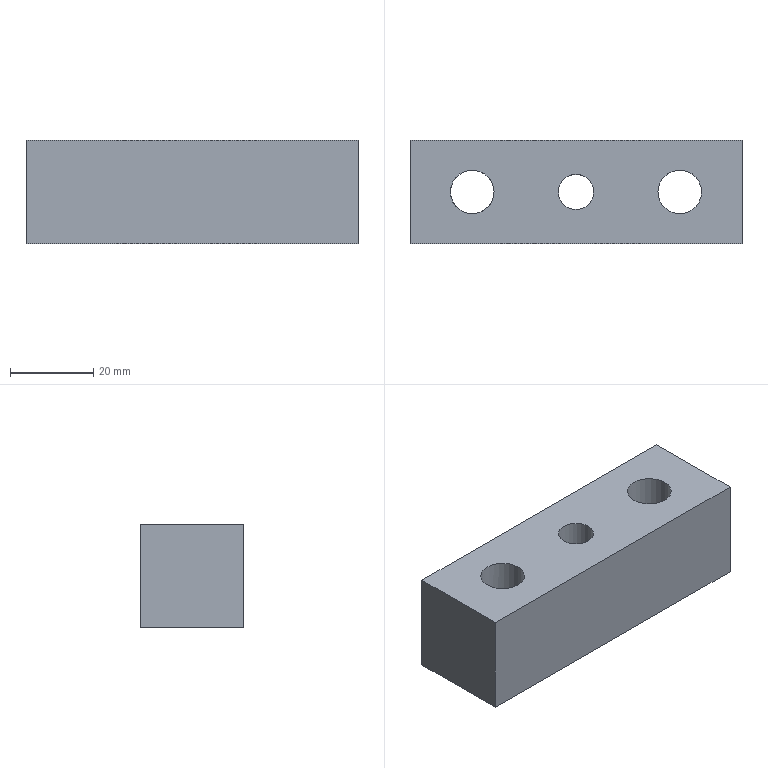Part | STEP file | 1_id1362_x_t | 1 solid | 15 faces | box 80 x 25 x 25 mm | volume 39657 mm3 | plane 9 | cylinder 6 | commonest cylinder face diameters 10.5 x2 17 x2 8.5 x1 11 x1
STEP:
#1=CARTESIAN_POINT('',(0.,0.,0.));
#2=DIRECTION('',(0.,0.,1.));
#3=DIRECTION('',(1.,0.,0.));
#4=AXIS2_PLACEMENT_3D('',#1,#2,#3);
#5=CARTESIAN_POINT('',(752.176,377.474,113.61));
#6=VERTEX_POINT('',#5);
#7=CARTESIAN_POINT('',(747.926,377.474,113.61));
#8=DIRECTION('',(0.,0.,-1.));
#9=DIRECTION('',(1.,0.,0.));
#10=AXIS2_PLACEMENT_3D('',#7,#8,#9);
#11=CIRCLE('',#10,4.25);
#12=CARTESIAN_POINT('',(747.926,377.474,117.86));
#13=DIRECTION('',(0.,0.,1.));
#14=DIRECTION('',(1.,0.,0.));
#15=AXIS2_PLACEMENT_3D('',#12,#13,#14);
#16=CYLINDRICAL_SURFACE('',#15,4.25);
#17=CARTESIAN_POINT('',(6.283,-4.25));
#18=DIRECTION('',(-1.,0.));
#19=VECTOR('',#18,1.);
#20=LINE('',#17,#19);
#21=(GEOMETRIC_REPRESENTATION_CONTEXT(2)PARAMETRIC_REPRESENTATION_CONTEXT()REPRESENTATION_CONTEXT('',''));
#22=DEFINITIONAL_REPRESENTATION('',(#20),#21);
#23=PCURVE('',#16,#22);
#24=CARTESIAN_POINT('',(707.926,389.974,113.61));
#25=DIRECTION('',(0.,0.,-1.));
#26=DIRECTION('',(-1.,0.,0.));
#27=AXIS2_PLACEMENT_3D('',#24,#25,#26);
#28=PLANE('',#27);
#29=CARTESIAN_POINT('',(-40.,-12.5));
#30=DIRECTION('',(-1.,0.));
#31=AXIS2_PLACEMENT_2D('',#29,#30);
#32=CIRCLE('',#31,4.25);
#33=(GEOMETRIC_REPRESENTATION_CONTEXT(2)PARAMETRIC_REPRESENTATION_CONTEXT()REPRESENTATION_CONTEXT('',''));
#34=DEFINITIONAL_REPRESENTATION('',(#32),#33);
#35=PCURVE('',#28,#34);
#36=SURFACE_CURVE('',#11,(#23,#35),.PCURVE_S1.);
#37=EDGE_CURVE('',#6,#6,#36,.T.);
#38=ORIENTED_EDGE('',*,*,#37,.T.);
#39=CARTESIAN_POINT('',(752.176,377.474,98.61));
#40=VERTEX_POINT('',#39);
#41=CARTESIAN_POINT('',(752.176,377.474,98.61));
#42=CARTESIAN_POINT('',(752.176,377.474,113.61));
#43=B_SPLINE_CURVE_WITH_KNOTS('',1,(#41,#42),.UNSPECIFIED.,.F.,.F.,(2,2),(-19.25,-4.25),.PIECEWISE_BEZIER_KNOTS.);
#44=CARTESIAN_POINT('',(0.,0.));
#45=DIRECTION('',(0.,1.));
#46=VECTOR('',#45,1.);
#47=LINE('',#44,#46);
#48=(GEOMETRIC_REPRESENTATION_CONTEXT(2)PARAMETRIC_REPRESENTATION_CONTEXT()REPRESENTATION_CONTEXT('',''));
#49=DEFINITIONAL_REPRESENTATION('',(#47),#48);
#50=PCURVE('',#16,#49);
#51=CARTESIAN_POINT('',(6.283,0.));
#52=DIRECTION('',(0.,1.));
#53=VECTOR('',#52,1.);
#54=LINE('',#51,#53);
#55=(GEOMETRIC_REPRESENTATION_CONTEXT(2)PARAMETRIC_REPRESENTATION_CONTEXT()REPRESENTATION_CONTEXT('',''));
#56=DEFINITIONAL_REPRESENTATION('',(#54),#55);
#57=PCURVE('',#16,#56);
#58=SEAM_CURVE('',#43,(#50,#57),.PCURVE_S1.);
#59=EDGE_CURVE('',#40,#6,#58,.T.);
#60=ORIENTED_EDGE('',*,*,#59,.F.);
#61=CARTESIAN_POINT('',(743.676,377.474,98.61));
#62=VERTEX_POINT('',#61);
#63=CARTESIAN_POINT('',(747.926,377.474,98.61));
#64=DIRECTION('',(0.,0.,1.));
#65=DIRECTION('',(-1.,0.,0.));
#66=AXIS2_PLACEMENT_3D('',#63,#64,#65);
#67=CIRCLE('',#66,4.25);
#68=CARTESIAN_POINT('',(-3.142,-19.25));
#69=DIRECTION('',(1.,0.));
#70=VECTOR('',#69,1.);
#71=LINE('',#68,#70);
#72=(GEOMETRIC_REPRESENTATION_CONTEXT(2)PARAMETRIC_REPRESENTATION_CONTEXT()REPRESENTATION_CONTEXT('',''));
#73=DEFINITIONAL_REPRESENTATION('',(#71),#72);
#74=PCURVE('',#16,#73);
#75=CARTESIAN_POINT('',(747.926,377.474,98.61));
#76=DIRECTION('',(0.,0.,-1.));
#77=DIRECTION('',(-1.,0.,0.));
#78=AXIS2_PLACEMENT_3D('',#75,#76,#77);
#79=PLANE('',#78);
#80=CARTESIAN_POINT('',(4.25,0.));
#81=CARTESIAN_POINT('',(4.25,-7.361));
#82=CARTESIAN_POINT('',(-2.125,-3.681));
#83=CARTESIAN_POINT('',(-8.5,0.));
#84=CARTESIAN_POINT('',(-2.125,3.681));
#85=CARTESIAN_POINT('',(4.25,7.361));
#86=CARTESIAN_POINT('',(4.25,0.));
#87=(BOUNDED_CURVE()B_SPLINE_CURVE(2,(#80,#81,#82,#83,#84,#85,#86),.UNSPECIFIED.,.T.,.F.)B_SPLINE_CURVE_WITH_KNOTS((1,2,2,2,2,1),(-2.094,0.,2.094,4.189,6.283,8.378),.UNSPECIFIED.)CURVE()GEOMETRIC_REPRESENTATION_ITEM()RATIONAL_B_SPLINE_CURVE((1.,0.5,1.,0.5,1.,0.5,1.))REPRESENTATION_ITEM(''));
#88=(GEOMETRIC_REPRESENTATION_CONTEXT(2)PARAMETRIC_REPRESENTATION_CONTEXT()REPRESENTATION_CONTEXT('',''));
#89=DEFINITIONAL_REPRESENTATION('',(#87),#88);
#90=PCURVE('',#79,#89);
#91=SURFACE_CURVE('',#67,(#74,#90),.PCURVE_S1.);
#92=EDGE_CURVE('',#40,#62,#91,.T.);
#93=ORIENTED_EDGE('',*,*,#92,.T.);
#94=CARTESIAN_POINT('',(747.926,377.474,98.61));
#95=DIRECTION('',(0.,0.,1.));
#96=DIRECTION('',(-1.,0.,0.));
#97=AXIS2_PLACEMENT_3D('',#94,#95,#96);
#98=CIRCLE('',#97,4.25);
#99=CARTESIAN_POINT('',(3.142,-19.25));
#100=DIRECTION('',(1.,0.));
#101=VECTOR('',#100,1.);
#102=LINE('',#99,#101);
#103=(GEOMETRIC_REPRESENTATION_CONTEXT(2)PARAMETRIC_REPRESENTATION_CONTEXT()REPRESENTATION_CONTEXT('',''));
#104=DEFINITIONAL_REPRESENTATION('',(#102),#103);
#105=PCURVE('',#16,#104);
#106=CARTESIAN_POINT('',(4.25,0.));
#107=CARTESIAN_POINT('',(4.25,-7.361));
#108=CARTESIAN_POINT('',(-2.125,-3.681));
#109=CARTESIAN_POINT('',(-8.5,0.));
#110=CARTESIAN_POINT('',(-2.125,3.681));
#111=CARTESIAN_POINT('',(4.25,7.361));
#112=CARTESIAN_POINT('',(4.25,0.));
#113=(BOUNDED_CURVE()B_SPLINE_CURVE(2,(#106,#107,#108,#109,#110,#111,#112),.UNSPECIFIED.,.T.,.F.)B_SPLINE_CURVE_WITH_KNOTS((1,2,2,2,2,1),(-2.094,0.,2.094,4.189,6.283,8.378),.UNSPECIFIED.)CURVE()GEOMETRIC_REPRESENTATION_ITEM()RATIONAL_B_SPLINE_CURVE((1.,0.5,1.,0.5,1.,0.5,1.))REPRESENTATION_ITEM(''));
#114=(GEOMETRIC_REPRESENTATION_CONTEXT(2)PARAMETRIC_REPRESENTATION_CONTEXT()REPRESENTATION_CONTEXT('',''));
#115=DEFINITIONAL_REPRESENTATION('',(#113),#114);
#116=PCURVE('',#79,#115);
#117=SURFACE_CURVE('',#98,(#105,#116),.PCURVE_S1.);
#118=EDGE_CURVE('',#62,#40,#117,.T.);
#119=ORIENTED_EDGE('',*,*,#118,.T.);
#120=ORIENTED_EDGE('',*,*,#59,.T.);
#121=EDGE_LOOP('',(#38,#60,#93,#119,#120));
#122=FACE_BOUND('',#121,.F.);
#123=ADVANCED_FACE('',(#122),#16,.F.);
#124=CARTESIAN_POINT('',(707.926,364.974,113.61));
#125=VERTEX_POINT('',#124);
#126=CARTESIAN_POINT('',(787.926,364.974,113.61));
#127=VERTEX_POINT('',#126);
#128=CARTESIAN_POINT('',(707.926,364.974,113.61));
#129=DIRECTION('',(1.,0.,0.));
#130=VECTOR('',#129,1.);
#131=LINE('',#128,#130);
#132=CARTESIAN_POINT('',(0.,-25.));
#133=DIRECTION('',(-1.,0.));
#134=VECTOR('',#133,1.);
#135=LINE('',#132,#134);
#136=(GEOMETRIC_REPRESENTATION_CONTEXT(2)PARAMETRIC_REPRESENTATION_CONTEXT()REPRESENTATION_CONTEXT('',''));
#137=DEFINITIONAL_REPRESENTATION('',(#135),#136);
#138=PCURVE('',#28,#137);
#139=CARTESIAN_POINT('',(787.926,364.974,113.61));
#140=DIRECTION('',(0.,-1.,0.));
#141=DIRECTION('',(-1.,0.,0.));
#142=AXIS2_PLACEMENT_3D('',#139,#140,#141);
#143=PLANE('',#142);
#144=CARTESIAN_POINT('',(80.,0.));
#145=DIRECTION('',(-1.,0.));
#146=VECTOR('',#145,1.);
#147=LINE('',#144,#146);
#148=(GEOMETRIC_REPRESENTATION_CONTEXT(2)PARAMETRIC_REPRESENTATION_CONTEXT()REPRESENTATION_CONTEXT('',''));
#149=DEFINITIONAL_REPRESENTATION('',(#147),#148);
#150=PCURVE('',#143,#149);
#151=SURFACE_CURVE('',#131,(#138,#150),.PCURVE_S1.);
#152=EDGE_CURVE('',#125,#127,#151,.T.);
#153=ORIENTED_EDGE('',*,*,#152,.T.);
#154=CARTESIAN_POINT('',(787.926,389.974,113.61));
#155=VERTEX_POINT('',#154);
#156=CARTESIAN_POINT('',(787.926,364.974,113.61));
#157=DIRECTION('',(0.,1.,0.));
#158=VECTOR('',#157,1.);
#159=LINE('',#156,#158);
#160=CARTESIAN_POINT('',(-80.,-25.));
#161=DIRECTION('',(0.,1.));
#162=VECTOR('',#161,1.);
#163=LINE('',#160,#162);
#164=(GEOMETRIC_REPRESENTATION_CONTEXT(2)PARAMETRIC_REPRESENTATION_CONTEXT()REPRESENTATION_CONTEXT('',''));
#165=DEFINITIONAL_REPRESENTATION('',(#163),#164);
#166=PCURVE('',#28,#165);
#167=CARTESIAN_POINT('',(787.926,389.974,113.61));
#168=DIRECTION('',(1.,0.,0.));
#169=DIRECTION('',(0.,1.,0.));
#170=AXIS2_PLACEMENT_3D('',#167,#168,#169);
#171=PLANE('',#170);
#172=CARTESIAN_POINT('',(-25.,0.));
#173=DIRECTION('',(1.,0.));
#174=VECTOR('',#173,1.);
#175=LINE('',#172,#174);
#176=(GEOMETRIC_REPRESENTATION_CONTEXT(2)PARAMETRIC_REPRESENTATION_CONTEXT()REPRESENTATION_CONTEXT('',''));
#177=DEFINITIONAL_REPRESENTATION('',(#175),#176);
#178=PCURVE('',#171,#177);
#179=SURFACE_CURVE('',#159,(#166,#178),.PCURVE_S1.);
#180=EDGE_CURVE('',#127,#155,#179,.T.);
#181=ORIENTED_EDGE('',*,*,#180,.T.);
#182=CARTESIAN_POINT('',(707.926,389.974,113.61));
#183=VERTEX_POINT('',#182);
#184=CARTESIAN_POINT('',(787.926,389.974,113.61));
#185=DIRECTION('',(-1.,0.,0.));
#186=VECTOR('',#185,1.);
#187=LINE('',#184,#186);
#188=CARTESIAN_POINT('',(-80.,0.));
#189=DIRECTION('',(1.,0.));
#190=VECTOR('',#189,1.);
#191=LINE('',#188,#190);
#192=(GEOMETRIC_REPRESENTATION_CONTEXT(2)PARAMETRIC_REPRESENTATION_CONTEXT()REPRESENTATION_CONTEXT('',''));
#193=DEFINITIONAL_REPRESENTATION('',(#191),#192);
#194=PCURVE('',#28,#193);
#195=CARTESIAN_POINT('',(707.926,389.974,113.61));
#196=DIRECTION('',(0.,1.,0.));
#197=DIRECTION('',(0.,0.,-1.));
#198=AXIS2_PLACEMENT_3D('',#195,#196,#197);
#199=PLANE('',#198);
#200=CARTESIAN_POINT('',(0.,-80.));
#201=DIRECTION('',(0.,1.));
#202=VECTOR('',#201,1.);
#203=LINE('',#200,#202);
#204=(GEOMETRIC_REPRESENTATION_CONTEXT(2)PARAMETRIC_REPRESENTATION_CONTEXT()REPRESENTATION_CONTEXT('',''));
#205=DEFINITIONAL_REPRESENTATION('',(#203),#204);
#206=PCURVE('',#199,#205);
#207=SURFACE_CURVE('',#187,(#194,#206),.PCURVE_S1.);
#208=EDGE_CURVE('',#155,#183,#207,.T.);
#209=ORIENTED_EDGE('',*,*,#208,.T.);
#210=CARTESIAN_POINT('',(707.926,389.974,113.61));
#211=DIRECTION('',(0.,-1.,0.));
#212=VECTOR('',#211,1.);
#213=LINE('',#210,#212);
#214=CARTESIAN_POINT('',(0.,0.));
#215=DIRECTION('',(0.,-1.));
#216=VECTOR('',#215,1.);
#217=LINE('',#214,#216);
#218=(GEOMETRIC_REPRESENTATION_CONTEXT(2)PARAMETRIC_REPRESENTATION_CONTEXT()REPRESENTATION_CONTEXT('',''));
#219=DEFINITIONAL_REPRESENTATION('',(#217),#218);
#220=PCURVE('',#28,#219);
#221=CARTESIAN_POINT('',(707.926,364.974,113.61));
#222=DIRECTION('',(-1.,0.,0.));
#223=DIRECTION('',(0.,0.,1.));
#224=AXIS2_PLACEMENT_3D('',#221,#222,#223);
#225=PLANE('',#224);
#226=CARTESIAN_POINT('',(0.,25.));
#227=DIRECTION('',(0.,-1.));
#228=VECTOR('',#227,1.);
#229=LINE('',#226,#228);
#230=(GEOMETRIC_REPRESENTATION_CONTEXT(2)PARAMETRIC_REPRESENTATION_CONTEXT()REPRESENTATION_CONTEXT('',''));
#231=DEFINITIONAL_REPRESENTATION('',(#229),#230);
#232=PCURVE('',#225,#231);
#233=SURFACE_CURVE('',#213,(#220,#232),.PCURVE_S1.);
#234=EDGE_CURVE('',#183,#125,#233,.T.);
#235=ORIENTED_EDGE('',*,*,#234,.T.);
#236=EDGE_LOOP('',(#153,#181,#209,#235));
#237=FACE_BOUND('',#236,.T.);
#238=CARTESIAN_POINT('',(728.176,377.474,113.61));
#239=VERTEX_POINT('',#238);
#240=CARTESIAN_POINT('',(722.926,377.474,113.61));
#241=DIRECTION('',(0.,0.,-1.));
#242=DIRECTION('',(1.,0.,0.));
#243=AXIS2_PLACEMENT_3D('',#240,#241,#242);
#244=CIRCLE('',#243,5.25);
#245=CARTESIAN_POINT('',(-15.,-12.5));
#246=DIRECTION('',(-1.,0.));
#247=AXIS2_PLACEMENT_2D('',#245,#246);
#248=CIRCLE('',#247,5.25);
#249=(GEOMETRIC_REPRESENTATION_CONTEXT(2)PARAMETRIC_REPRESENTATION_CONTEXT()REPRESENTATION_CONTEXT('',''));
#250=DEFINITIONAL_REPRESENTATION('',(#248),#249);
#251=PCURVE('',#28,#250);
#252=CARTESIAN_POINT('',(722.926,377.474,113.86));
#253=DIRECTION('',(0.,0.,1.));
#254=DIRECTION('',(0.,1.,0.));
#255=AXIS2_PLACEMENT_3D('',#252,#253,#254);
#256=CYLINDRICAL_SURFACE('',#255,5.25);
#257=CARTESIAN_POINT('',(10.996,-0.25));
#258=DIRECTION('',(-1.,0.));
#259=VECTOR('',#258,1.);
#260=LINE('',#257,#259);
#261=(GEOMETRIC_REPRESENTATION_CONTEXT(2)PARAMETRIC_REPRESENTATION_CONTEXT()REPRESENTATION_CONTEXT('',''));
#262=DEFINITIONAL_REPRESENTATION('',(#260),#261);
#263=PCURVE('',#256,#262);
#264=SURFACE_CURVE('',#244,(#251,#263),.PCURVE_S1.);
#265=EDGE_CURVE('',#239,#239,#264,.T.);
#266=ORIENTED_EDGE('',*,*,#265,.T.);
#267=EDGE_LOOP('',(#266));
#268=FACE_BOUND('',#267,.T.);
#269=ORIENTED_EDGE('',*,*,#37,.T.);
#270=EDGE_LOOP('',(#269));
#271=FACE_BOUND('',#270,.T.);
#272=CARTESIAN_POINT('',(778.176,377.474,113.61));
#273=VERTEX_POINT('',#272);
#274=CARTESIAN_POINT('',(772.926,377.474,113.61));
#275=DIRECTION('',(0.,0.,-1.));
#276=DIRECTION('',(1.,0.,0.));
#277=AXIS2_PLACEMENT_3D('',#274,#275,#276);
#278=CIRCLE('',#277,5.25);
#279=CARTESIAN_POINT('',(-65.,-12.5));
#280=DIRECTION('',(-1.,0.));
#281=AXIS2_PLACEMENT_2D('',#279,#280);
#282=CIRCLE('',#281,5.25);
#283=(GEOMETRIC_REPRESENTATION_CONTEXT(2)PARAMETRIC_REPRESENTATION_CONTEXT()REPRESENTATION_CONTEXT('',''));
#284=DEFINITIONAL_REPRESENTATION('',(#282),#283);
#285=PCURVE('',#28,#284);
#286=CARTESIAN_POINT('',(772.926,377.474,113.86));
#287=DIRECTION('',(0.,0.,1.));
#288=DIRECTION('',(0.,1.,0.));
#289=AXIS2_PLACEMENT_3D('',#286,#287,#288);
#290=CYLINDRICAL_SURFACE('',#289,5.25);
#291=CARTESIAN_POINT('',(10.996,-0.25));
#292=DIRECTION('',(-1.,0.));
#293=VECTOR('',#292,1.);
#294=LINE('',#291,#293);
#295=(GEOMETRIC_REPRESENTATION_CONTEXT(2)PARAMETRIC_REPRESENTATION_CONTEXT()REPRESENTATION_CONTEXT('',''));
#296=DEFINITIONAL_REPRESENTATION('',(#294),#295);
#297=PCURVE('',#290,#296);
#298=SURFACE_CURVE('',#278,(#285,#297),.PCURVE_S1.);
#299=EDGE_CURVE('',#273,#273,#298,.T.);
#300=ORIENTED_EDGE('',*,*,#299,.T.);
#301=EDGE_LOOP('',(#300));
#302=FACE_BOUND('',#301,.T.);
#303=ADVANCED_FACE('',(#237,#268,#271,#302),#28,.F.);
#304=ORIENTED_EDGE('',*,*,#265,.T.);
#305=CARTESIAN_POINT('',(728.176,377.474,103.61));
#306=VERTEX_POINT('',#305);
#307=CARTESIAN_POINT('',(728.176,377.474,103.61));
#308=CARTESIAN_POINT('',(728.176,377.474,113.61));
#309=B_SPLINE_CURVE_WITH_KNOTS('',1,(#307,#308),.UNSPECIFIED.,.F.,.F.,(2,2),(-10.25,-0.25),.PIECEWISE_BEZIER_KNOTS.);
#310=CARTESIAN_POINT('',(4.712,0.));
#311=DIRECTION('',(0.,1.));
#312=VECTOR('',#311,1.);
#313=LINE('',#310,#312);
#314=(GEOMETRIC_REPRESENTATION_CONTEXT(2)PARAMETRIC_REPRESENTATION_CONTEXT()REPRESENTATION_CONTEXT('',''));
#315=DEFINITIONAL_REPRESENTATION('',(#313),#314);
#316=PCURVE('',#256,#315);
#317=CARTESIAN_POINT('',(10.996,0.));
#318=DIRECTION('',(0.,1.));
#319=VECTOR('',#318,1.);
#320=LINE('',#317,#319);
#321=(GEOMETRIC_REPRESENTATION_CONTEXT(2)PARAMETRIC_REPRESENTATION_CONTEXT()REPRESENTATION_CONTEXT('',''));
#322=DEFINITIONAL_REPRESENTATION('',(#320),#321);
#323=PCURVE('',#256,#322);
#324=SEAM_CURVE('',#309,(#316,#323),.PCURVE_S1.);
#325=EDGE_CURVE('',#306,#239,#324,.T.);
#326=ORIENTED_EDGE('',*,*,#325,.F.);
#327=CARTESIAN_POINT('',(722.926,372.224,103.61));
#328=VERTEX_POINT('',#327);
#329=CARTESIAN_POINT('',(722.926,377.474,103.61));
#330=DIRECTION('',(0.,0.,1.));
#331=DIRECTION('',(0.,-1.,0.));
#332=AXIS2_PLACEMENT_3D('',#329,#330,#331);
#333=CIRCLE('',#332,5.25);
#334=CARTESIAN_POINT('',(3.142,-10.25));
#335=DIRECTION('',(1.,0.));
#336=VECTOR('',#335,1.);
#337=LINE('',#334,#336);
#338=(GEOMETRIC_REPRESENTATION_CONTEXT(2)PARAMETRIC_REPRESENTATION_CONTEXT()REPRESENTATION_CONTEXT('',''));
#339=DEFINITIONAL_REPRESENTATION('',(#337),#338);
#340=PCURVE('',#256,#339);
#341=CARTESIAN_POINT('',(722.926,377.474,103.61));
#342=DIRECTION('',(0.,0.,1.));
#343=DIRECTION('',(0.,-1.,0.));
#344=AXIS2_PLACEMENT_3D('',#341,#342,#343);
#345=PLANE('',#344);
#346=CARTESIAN_POINT('',(0.,0.));
#347=DIRECTION('',(1.,0.));
#348=AXIS2_PLACEMENT_2D('',#346,#347);
#349=CIRCLE('',#348,5.25);
#350=(GEOMETRIC_REPRESENTATION_CONTEXT(2)PARAMETRIC_REPRESENTATION_CONTEXT()REPRESENTATION_CONTEXT('',''));
#351=DEFINITIONAL_REPRESENTATION('',(#349),#350);
#352=PCURVE('',#345,#351);
#353=SURFACE_CURVE('',#333,(#340,#352),.PCURVE_S1.);
#354=EDGE_CURVE('',#306,#328,#353,.T.);
#355=ORIENTED_EDGE('',*,*,#354,.T.);
#356=CARTESIAN_POINT('',(722.926,377.474,103.61));
#357=DIRECTION('',(0.,0.,1.));
#358=DIRECTION('',(0.,-1.,0.));
#359=AXIS2_PLACEMENT_3D('',#356,#357,#358);
#360=CIRCLE('',#359,5.25);
#361=CARTESIAN_POINT('',(9.425,-10.25));
#362=DIRECTION('',(1.,0.));
#363=VECTOR('',#362,1.);
#364=LINE('',#361,#363);
#365=(GEOMETRIC_REPRESENTATION_CONTEXT(2)PARAMETRIC_REPRESENTATION_CONTEXT()REPRESENTATION_CONTEXT('',''));
#366=DEFINITIONAL_REPRESENTATION('',(#364),#365);
#367=PCURVE('',#256,#366);
#368=CARTESIAN_POINT('',(0.,0.));
#369=DIRECTION('',(1.,0.));
#370=AXIS2_PLACEMENT_2D('',#368,#369);
#371=CIRCLE('',#370,5.25);
#372=(GEOMETRIC_REPRESENTATION_CONTEXT(2)PARAMETRIC_REPRESENTATION_CONTEXT()REPRESENTATION_CONTEXT('',''));
#373=DEFINITIONAL_REPRESENTATION('',(#371),#372);
#374=PCURVE('',#345,#373);
#375=SURFACE_CURVE('',#360,(#367,#374),.PCURVE_S1.);
#376=EDGE_CURVE('',#328,#306,#375,.T.);
#377=ORIENTED_EDGE('',*,*,#376,.T.);
#378=ORIENTED_EDGE('',*,*,#325,.T.);
#379=EDGE_LOOP('',(#304,#326,#355,#377,#378));
#380=FACE_BOUND('',#379,.F.);
#381=ADVANCED_FACE('',(#380),#256,.F.);
#382=CARTESIAN_POINT('',(722.926,368.974,103.61));
#383=VERTEX_POINT('',#382);
#384=CARTESIAN_POINT('',(722.926,385.974,103.61));
#385=VERTEX_POINT('',#384);
#386=CARTESIAN_POINT('',(722.926,377.474,103.61));
#387=DIRECTION('',(0.,0.,-1.));
#388=DIRECTION('',(0.,-1.,0.));
#389=AXIS2_PLACEMENT_3D('',#386,#387,#388);
#390=CIRCLE('',#389,8.5);
#391=CARTESIAN_POINT('',(8.5,0.));
#392=CARTESIAN_POINT('',(8.5,-14.722));
#393=CARTESIAN_POINT('',(-4.25,-7.361));
#394=CARTESIAN_POINT('',(-17.,0.));
#395=CARTESIAN_POINT('',(-4.25,7.361));
#396=CARTESIAN_POINT('',(8.5,14.722));
#397=CARTESIAN_POINT('',(8.5,0.));
#398=(BOUNDED_CURVE()B_SPLINE_CURVE(2,(#391,#392,#393,#394,#395,#396,#397),.UNSPECIFIED.,.T.,.F.)B_SPLINE_CURVE_WITH_KNOTS((1,2,2,2,2,1),(-2.094,0.,2.094,4.189,6.283,8.378),.UNSPECIFIED.)CURVE()GEOMETRIC_REPRESENTATION_ITEM()RATIONAL_B_SPLINE_CURVE((1.,0.5,1.,0.5,1.,0.5,1.))REPRESENTATION_ITEM(''));
#399=(GEOMETRIC_REPRESENTATION_CONTEXT(2)PARAMETRIC_REPRESENTATION_CONTEXT()REPRESENTATION_CONTEXT('',''));
#400=DEFINITIONAL_REPRESENTATION('',(#398),#399);
#401=PCURVE('',#345,#400);
#402=CARTESIAN_POINT('',(722.926,377.474,103.61));
#403=DIRECTION('',(0.,0.,1.));
#404=DIRECTION('',(0.,1.,0.));
#405=AXIS2_PLACEMENT_3D('',#402,#403,#404);
#406=CYLINDRICAL_SURFACE('',#405,8.5);
#407=CARTESIAN_POINT('',(3.142,0.));
#408=DIRECTION('',(-1.,0.));
#409=VECTOR('',#408,1.);
#410=LINE('',#407,#409);
#411=(GEOMETRIC_REPRESENTATION_CONTEXT(2)PARAMETRIC_REPRESENTATION_CONTEXT()REPRESENTATION_CONTEXT('',''));
#412=DEFINITIONAL_REPRESENTATION('',(#410),#411);
#413=PCURVE('',#406,#412);
#414=SURFACE_CURVE('',#390,(#401,#413),.PCURVE_S1.);
#415=EDGE_CURVE('',#383,#385,#414,.T.);
#416=ORIENTED_EDGE('',*,*,#415,.T.);
#417=CARTESIAN_POINT('',(722.926,377.474,103.61));
#418=DIRECTION('',(0.,0.,-1.));
#419=DIRECTION('',(0.,-1.,0.));
#420=AXIS2_PLACEMENT_3D('',#417,#418,#419);
#421=CIRCLE('',#420,8.5);
#422=CARTESIAN_POINT('',(8.5,0.));
#423=CARTESIAN_POINT('',(8.5,-14.722));
#424=CARTESIAN_POINT('',(-4.25,-7.361));
#425=CARTESIAN_POINT('',(-17.,0.));
#426=CARTESIAN_POINT('',(-4.25,7.361));
#427=CARTESIAN_POINT('',(8.5,14.722));
#428=CARTESIAN_POINT('',(8.5,0.));
#429=(BOUNDED_CURVE()B_SPLINE_CURVE(2,(#422,#423,#424,#425,#426,#427,#428),.UNSPECIFIED.,.T.,.F.)B_SPLINE_CURVE_WITH_KNOTS((1,2,2,2,2,1),(-2.094,0.,2.094,4.189,6.283,8.378),.UNSPECIFIED.)CURVE()GEOMETRIC_REPRESENTATION_ITEM()RATIONAL_B_SPLINE_CURVE((1.,0.5,1.,0.5,1.,0.5,1.))REPRESENTATION_ITEM(''));
#430=(GEOMETRIC_REPRESENTATION_CONTEXT(2)PARAMETRIC_REPRESENTATION_CONTEXT()REPRESENTATION_CONTEXT('',''));
#431=DEFINITIONAL_REPRESENTATION('',(#429),#430);
#432=PCURVE('',#345,#431);
#433=CARTESIAN_POINT('',(9.425,0.));
#434=DIRECTION('',(-1.,0.));
#435=VECTOR('',#434,1.);
#436=LINE('',#433,#435);
#437=(GEOMETRIC_REPRESENTATION_CONTEXT(2)PARAMETRIC_REPRESENTATION_CONTEXT()REPRESENTATION_CONTEXT('',''));
#438=DEFINITIONAL_REPRESENTATION('',(#436),#437);
#439=PCURVE('',#406,#438);
#440=SURFACE_CURVE('',#421,(#432,#439),.PCURVE_S1.);
#441=EDGE_CURVE('',#385,#383,#440,.T.);
#442=ORIENTED_EDGE('',*,*,#441,.T.);
#443=EDGE_LOOP('',(#416,#442));
#444=FACE_BOUND('',#443,.T.);
#445=ORIENTED_EDGE('',*,*,#376,.T.);
#446=ORIENTED_EDGE('',*,*,#354,.T.);
#447=EDGE_LOOP('',(#445,#446));
#448=FACE_BOUND('',#447,.T.);
#449=ADVANCED_FACE('',(#444,#448),#345,.F.);
#450=ORIENTED_EDGE('',*,*,#415,.T.);
#451=CARTESIAN_POINT('',(722.926,385.974,88.61));
#452=VERTEX_POINT('',#451);
#453=CARTESIAN_POINT('',(722.926,385.974,88.61));
#454=CARTESIAN_POINT('',(722.926,385.974,103.61));
#455=B_SPLINE_CURVE_WITH_KNOTS('',1,(#453,#454),.UNSPECIFIED.,.F.,.F.,(2,2),(-15.,0.),.PIECEWISE_BEZIER_KNOTS.);
#456=CARTESIAN_POINT('',(0.,0.));
#457=DIRECTION('',(0.,1.));
#458=VECTOR('',#457,1.);
#459=LINE('',#456,#458);
#460=(GEOMETRIC_REPRESENTATION_CONTEXT(2)PARAMETRIC_REPRESENTATION_CONTEXT()REPRESENTATION_CONTEXT('',''));
#461=DEFINITIONAL_REPRESENTATION('',(#459),#460);
#462=PCURVE('',#406,#461);
#463=CARTESIAN_POINT('',(6.283,0.));
#464=DIRECTION('',(0.,1.));
#465=VECTOR('',#464,1.);
#466=LINE('',#463,#465);
#467=(GEOMETRIC_REPRESENTATION_CONTEXT(2)PARAMETRIC_REPRESENTATION_CONTEXT()REPRESENTATION_CONTEXT('',''));
#468=DEFINITIONAL_REPRESENTATION('',(#466),#467);
#469=PCURVE('',#406,#468);
#470=SEAM_CURVE('',#455,(#462,#469),.PCURVE_S1.);
#471=EDGE_CURVE('',#452,#385,#470,.T.);
#472=ORIENTED_EDGE('',*,*,#471,.F.);
#473=CARTESIAN_POINT('',(722.926,377.474,88.61));
#474=DIRECTION('',(0.,0.,1.));
#475=DIRECTION('',(0.,1.,0.));
#476=AXIS2_PLACEMENT_3D('',#473,#474,#475);
#477=CIRCLE('',#476,8.5);
#478=CARTESIAN_POINT('',(0.,-15.));
#479=DIRECTION('',(1.,0.));
#480=VECTOR('',#479,1.);
#481=LINE('',#478,#480);
#482=(GEOMETRIC_REPRESENTATION_CONTEXT(2)PARAMETRIC_REPRESENTATION_CONTEXT()REPRESENTATION_CONTEXT('',''));
#483=DEFINITIONAL_REPRESENTATION('',(#481),#482);
#484=PCURVE('',#406,#483);
#485=CARTESIAN_POINT('',(707.926,389.974,88.61));
#486=DIRECTION('',(0.,0.,-1.));
#487=DIRECTION('',(-1.,0.,0.));
#488=AXIS2_PLACEMENT_3D('',#485,#486,#487);
#489=PLANE('',#488);
#490=CARTESIAN_POINT('',(-15.,-4.));
#491=CARTESIAN_POINT('',(-0.2776,-4.));
#492=CARTESIAN_POINT('',(-7.639,-16.75));
#493=CARTESIAN_POINT('',(-15.,-29.5));
#494=CARTESIAN_POINT('',(-22.361,-16.75));
#495=CARTESIAN_POINT('',(-29.722,-4.));
#496=CARTESIAN_POINT('',(-15.,-4.));
#497=(BOUNDED_CURVE()B_SPLINE_CURVE(2,(#490,#491,#492,#493,#494,#495,#496),.UNSPECIFIED.,.T.,.F.)B_SPLINE_CURVE_WITH_KNOTS((1,2,2,2,2,1),(-2.094,0.,2.094,4.189,6.283,8.378),.UNSPECIFIED.)CURVE()GEOMETRIC_REPRESENTATION_ITEM()RATIONAL_B_SPLINE_CURVE((1.,0.5,1.,0.5,1.,0.5,1.))REPRESENTATION_ITEM(''));
#498=(GEOMETRIC_REPRESENTATION_CONTEXT(2)PARAMETRIC_REPRESENTATION_CONTEXT()REPRESENTATION_CONTEXT('',''));
#499=DEFINITIONAL_REPRESENTATION('',(#497),#498);
#500=PCURVE('',#489,#499);
#501=SURFACE_CURVE('',#477,(#484,#500),.PCURVE_S1.);
#502=EDGE_CURVE('',#452,#452,#501,.T.);
#503=ORIENTED_EDGE('',*,*,#502,.T.);
#504=ORIENTED_EDGE('',*,*,#471,.T.);
#505=ORIENTED_EDGE('',*,*,#441,.T.);
#506=EDGE_LOOP('',(#450,#472,#503,#504,#505));
#507=FACE_BOUND('',#506,.F.);
#508=ADVANCED_FACE('',(#507),#406,.F.);
#509=CARTESIAN_POINT('',(787.926,389.974,88.61));
#510=VERTEX_POINT('',#509);
#511=CARTESIAN_POINT('',(707.926,389.974,88.61));
#512=VERTEX_POINT('',#511);
#513=CARTESIAN_POINT('',(787.926,389.974,88.61));
#514=DIRECTION('',(-1.,0.,0.));
#515=VECTOR('',#514,1.);
#516=LINE('',#513,#515);
#517=CARTESIAN_POINT('',(-80.,0.));
#518=DIRECTION('',(1.,0.));
#519=VECTOR('',#518,1.);
#520=LINE('',#517,#519);
#521=(GEOMETRIC_REPRESENTATION_CONTEXT(2)PARAMETRIC_REPRESENTATION_CONTEXT()REPRESENTATION_CONTEXT('',''));
#522=DEFINITIONAL_REPRESENTATION('',(#520),#521);
#523=PCURVE('',#489,#522);
#524=CARTESIAN_POINT('',(25.,-80.));
#525=DIRECTION('',(0.,1.));
#526=VECTOR('',#525,1.);
#527=LINE('',#524,#526);
#528=(GEOMETRIC_REPRESENTATION_CONTEXT(2)PARAMETRIC_REPRESENTATION_CONTEXT()REPRESENTATION_CONTEXT('',''));
#529=DEFINITIONAL_REPRESENTATION('',(#527),#528);
#530=PCURVE('',#199,#529);
#531=SURFACE_CURVE('',#516,(#523,#530),.PCURVE_S1.);
#532=EDGE_CURVE('',#510,#512,#531,.T.);
#533=ORIENTED_EDGE('',*,*,#532,.F.);
#534=CARTESIAN_POINT('',(787.926,364.974,88.61));
#535=VERTEX_POINT('',#534);
#536=CARTESIAN_POINT('',(787.926,364.974,88.61));
#537=DIRECTION('',(0.,1.,0.));
#538=VECTOR('',#537,1.);
#539=LINE('',#536,#538);
#540=CARTESIAN_POINT('',(-80.,-25.));
#541=DIRECTION('',(0.,1.));
#542=VECTOR('',#541,1.);
#543=LINE('',#540,#542);
#544=(GEOMETRIC_REPRESENTATION_CONTEXT(2)PARAMETRIC_REPRESENTATION_CONTEXT()REPRESENTATION_CONTEXT('',''));
#545=DEFINITIONAL_REPRESENTATION('',(#543),#544);
#546=PCURVE('',#489,#545);
#547=CARTESIAN_POINT('',(-25.,-25.));
#548=DIRECTION('',(1.,0.));
#549=VECTOR('',#548,1.);
#550=LINE('',#547,#549);
#551=(GEOMETRIC_REPRESENTATION_CONTEXT(2)PARAMETRIC_REPRESENTATION_CONTEXT()REPRESENTATION_CONTEXT('',''));
#552=DEFINITIONAL_REPRESENTATION('',(#550),#551);
#553=PCURVE('',#171,#552);
#554=SURFACE_CURVE('',#539,(#546,#553),.PCURVE_S1.);
#555=EDGE_CURVE('',#535,#510,#554,.T.);
#556=ORIENTED_EDGE('',*,*,#555,.F.);
#557=CARTESIAN_POINT('',(707.926,364.974,88.61));
#558=VERTEX_POINT('',#557);
#559=CARTESIAN_POINT('',(707.926,364.974,88.61));
#560=DIRECTION('',(1.,0.,0.));
#561=VECTOR('',#560,1.);
#562=LINE('',#559,#561);
#563=CARTESIAN_POINT('',(0.,-25.));
#564=DIRECTION('',(-1.,0.));
#565=VECTOR('',#564,1.);
#566=LINE('',#563,#565);
#567=(GEOMETRIC_REPRESENTATION_CONTEXT(2)PARAMETRIC_REPRESENTATION_CONTEXT()REPRESENTATION_CONTEXT('',''));
#568=DEFINITIONAL_REPRESENTATION('',(#566),#567);
#569=PCURVE('',#489,#568);
#570=CARTESIAN_POINT('',(80.,25.));
#571=DIRECTION('',(-1.,0.));
#572=VECTOR('',#571,1.);
#573=LINE('',#570,#572);
#574=(GEOMETRIC_REPRESENTATION_CONTEXT(2)PARAMETRIC_REPRESENTATION_CONTEXT()REPRESENTATION_CONTEXT('',''));
#575=DEFINITIONAL_REPRESENTATION('',(#573),#574);
#576=PCURVE('',#143,#575);
#577=SURFACE_CURVE('',#562,(#569,#576),.PCURVE_S1.);
#578=EDGE_CURVE('',#558,#535,#577,.T.);
#579=ORIENTED_EDGE('',*,*,#578,.F.);
#580=CARTESIAN_POINT('',(707.926,389.974,88.61));
#581=DIRECTION('',(0.,-1.,0.));
#582=VECTOR('',#581,1.);
#583=LINE('',#580,#582);
#584=CARTESIAN_POINT('',(0.,0.));
#585=DIRECTION('',(0.,-1.));
#586=VECTOR('',#585,1.);
#587=LINE('',#584,#586);
#588=(GEOMETRIC_REPRESENTATION_CONTEXT(2)PARAMETRIC_REPRESENTATION_CONTEXT()REPRESENTATION_CONTEXT('',''));
#589=DEFINITIONAL_REPRESENTATION('',(#587),#588);
#590=PCURVE('',#489,#589);
#591=CARTESIAN_POINT('',(-25.,25.));
#592=DIRECTION('',(0.,-1.));
#593=VECTOR('',#592,1.);
#594=LINE('',#591,#593);
#595=(GEOMETRIC_REPRESENTATION_CONTEXT(2)PARAMETRIC_REPRESENTATION_CONTEXT()REPRESENTATION_CONTEXT('',''));
#596=DEFINITIONAL_REPRESENTATION('',(#594),#595);
#597=PCURVE('',#225,#596);
#598=SURFACE_CURVE('',#583,(#590,#597),.PCURVE_S1.);
#599=EDGE_CURVE('',#512,#558,#598,.T.);
#600=ORIENTED_EDGE('',*,*,#599,.F.);
#601=EDGE_LOOP('',(#533,#556,#579,#600));
#602=FACE_BOUND('',#601,.T.);
#603=CARTESIAN_POINT('',(753.426,377.474,88.61));
#604=VERTEX_POINT('',#603);
#605=CARTESIAN_POINT('',(742.426,377.474,88.61));
#606=VERTEX_POINT('',#605);
#607=CARTESIAN_POINT('',(747.926,377.474,88.61));
#608=DIRECTION('',(0.,0.,1.));
#609=DIRECTION('',(1.,0.,0.));
#610=AXIS2_PLACEMENT_3D('',#607,#608,#609);
#611=CIRCLE('',#610,5.5);
#612=CARTESIAN_POINT('',(-45.5,-12.5));
#613=CARTESIAN_POINT('',(-45.5,-2.974));
#614=CARTESIAN_POINT('',(-37.25,-7.737));
#615=CARTESIAN_POINT('',(-29.,-12.5));
#616=CARTESIAN_POINT('',(-37.25,-17.263));
#617=CARTESIAN_POINT('',(-45.5,-22.026));
#618=CARTESIAN_POINT('',(-45.5,-12.5));
#619=(BOUNDED_CURVE()B_SPLINE_CURVE(2,(#612,#613,#614,#615,#616,#617,#618),.UNSPECIFIED.,.T.,.F.)B_SPLINE_CURVE_WITH_KNOTS((1,2,2,2,2,1),(-2.094,0.,2.094,4.189,6.283,8.378),.UNSPECIFIED.)CURVE()GEOMETRIC_REPRESENTATION_ITEM()RATIONAL_B_SPLINE_CURVE((1.,0.5,1.,0.5,1.,0.5,1.))REPRESENTATION_ITEM(''));
#620=(GEOMETRIC_REPRESENTATION_CONTEXT(2)PARAMETRIC_REPRESENTATION_CONTEXT()REPRESENTATION_CONTEXT('',''));
#621=DEFINITIONAL_REPRESENTATION('',(#619),#620);
#622=PCURVE('',#489,#621);
#623=CARTESIAN_POINT('',(747.926,377.474,98.61));
#624=DIRECTION('',(0.,0.,-1.));
#625=DIRECTION('',(-1.,0.,0.));
#626=AXIS2_PLACEMENT_3D('',#623,#624,#625);
#627=CYLINDRICAL_SURFACE('',#626,5.5);
#628=CARTESIAN_POINT('',(3.142,10.));
#629=DIRECTION('',(-1.,0.));
#630=VECTOR('',#629,1.);
#631=LINE('',#628,#630);
#632=(GEOMETRIC_REPRESENTATION_CONTEXT(2)PARAMETRIC_REPRESENTATION_CONTEXT()REPRESENTATION_CONTEXT('',''));
#633=DEFINITIONAL_REPRESENTATION('',(#631),#632);
#634=PCURVE('',#627,#633);
#635=SURFACE_CURVE('',#611,(#622,#634),.PCURVE_S1.);
#636=EDGE_CURVE('',#604,#606,#635,.T.);
#637=ORIENTED_EDGE('',*,*,#636,.T.);
#638=CARTESIAN_POINT('',(747.926,377.474,88.61));
#639=DIRECTION('',(0.,0.,1.));
#640=DIRECTION('',(1.,0.,0.));
#641=AXIS2_PLACEMENT_3D('',#638,#639,#640);
#642=CIRCLE('',#641,5.5);
#643=CARTESIAN_POINT('',(-45.5,-12.5));
#644=CARTESIAN_POINT('',(-45.5,-2.974));
#645=CARTESIAN_POINT('',(-37.25,-7.737));
#646=CARTESIAN_POINT('',(-29.,-12.5));
#647=CARTESIAN_POINT('',(-37.25,-17.263));
#648=CARTESIAN_POINT('',(-45.5,-22.026));
#649=CARTESIAN_POINT('',(-45.5,-12.5));
#650=(BOUNDED_CURVE()B_SPLINE_CURVE(2,(#643,#644,#645,#646,#647,#648,#649),.UNSPECIFIED.,.T.,.F.)B_SPLINE_CURVE_WITH_KNOTS((1,2,2,2,2,1),(-2.094,0.,2.094,4.189,6.283,8.378),.UNSPECIFIED.)CURVE()GEOMETRIC_REPRESENTATION_ITEM()RATIONAL_B_SPLINE_CURVE((1.,0.5,1.,0.5,1.,0.5,1.))REPRESENTATION_ITEM(''));
#651=(GEOMETRIC_REPRESENTATION_CONTEXT(2)PARAMETRIC_REPRESENTATION_CONTEXT()REPRESENTATION_CONTEXT('',''));
#652=DEFINITIONAL_REPRESENTATION('',(#650),#651);
#653=PCURVE('',#489,#652);
#654=CARTESIAN_POINT('',(9.425,10.));
#655=DIRECTION('',(-1.,0.));
#656=VECTOR('',#655,1.);
#657=LINE('',#654,#656);
#658=(GEOMETRIC_REPRESENTATION_CONTEXT(2)PARAMETRIC_REPRESENTATION_CONTEXT()REPRESENTATION_CONTEXT('',''));
#659=DEFINITIONAL_REPRESENTATION('',(#657),#658);
#660=PCURVE('',#627,#659);
#661=SURFACE_CURVE('',#642,(#653,#660),.PCURVE_S1.);
#662=EDGE_CURVE('',#606,#604,#661,.T.);
#663=ORIENTED_EDGE('',*,*,#662,.T.);
#664=EDGE_LOOP('',(#637,#663));
#665=FACE_BOUND('',#664,.T.);
#666=ORIENTED_EDGE('',*,*,#502,.T.);
#667=EDGE_LOOP('',(#666));
#668=FACE_BOUND('',#667,.T.);
#669=CARTESIAN_POINT('',(772.926,368.974,88.61));
#670=VERTEX_POINT('',#669);
#671=CARTESIAN_POINT('',(772.926,385.974,88.61));
#672=VERTEX_POINT('',#671);
#673=CARTESIAN_POINT('',(772.926,377.474,88.61));
#674=DIRECTION('',(0.,0.,1.));
#675=DIRECTION('',(0.,-1.,0.));
#676=AXIS2_PLACEMENT_3D('',#673,#674,#675);
#677=CIRCLE('',#676,8.5);
#678=CARTESIAN_POINT('',(-65.,-21.));
#679=CARTESIAN_POINT('',(-79.722,-21.));
#680=CARTESIAN_POINT('',(-72.361,-8.25));
#681=CARTESIAN_POINT('',(-65.,4.5));
#682=CARTESIAN_POINT('',(-57.639,-8.25));
#683=CARTESIAN_POINT('',(-50.278,-21.));
#684=CARTESIAN_POINT('',(-65.,-21.));
#685=(BOUNDED_CURVE()B_SPLINE_CURVE(2,(#678,#679,#680,#681,#682,#683,#684),.UNSPECIFIED.,.T.,.F.)B_SPLINE_CURVE_WITH_KNOTS((1,2,2,2,2,1),(-2.094,0.,2.094,4.189,6.283,8.378),.UNSPECIFIED.)CURVE()GEOMETRIC_REPRESENTATION_ITEM()RATIONAL_B_SPLINE_CURVE((1.,0.5,1.,0.5,1.,0.5,1.))REPRESENTATION_ITEM(''));
#686=(GEOMETRIC_REPRESENTATION_CONTEXT(2)PARAMETRIC_REPRESENTATION_CONTEXT()REPRESENTATION_CONTEXT('',''));
#687=DEFINITIONAL_REPRESENTATION('',(#685),#686);
#688=PCURVE('',#489,#687);
#689=CARTESIAN_POINT('',(772.926,377.474,103.61));
#690=DIRECTION('',(0.,0.,1.));
#691=DIRECTION('',(0.,1.,0.));
#692=AXIS2_PLACEMENT_3D('',#689,#690,#691);
#693=CYLINDRICAL_SURFACE('',#692,8.5);
#694=CARTESIAN_POINT('',(3.142,-15.));
#695=DIRECTION('',(1.,0.));
#696=VECTOR('',#695,1.);
#697=LINE('',#694,#696);
#698=(GEOMETRIC_REPRESENTATION_CONTEXT(2)PARAMETRIC_REPRESENTATION_CONTEXT()REPRESENTATION_CONTEXT('',''));
#699=DEFINITIONAL_REPRESENTATION('',(#697),#698);
#700=PCURVE('',#693,#699);
#701=SURFACE_CURVE('',#677,(#688,#700),.PCURVE_S1.);
#702=EDGE_CURVE('',#670,#672,#701,.T.);
#703=ORIENTED_EDGE('',*,*,#702,.T.);
#704=CARTESIAN_POINT('',(772.926,377.474,88.61));
#705=DIRECTION('',(0.,0.,1.));
#706=DIRECTION('',(0.,-1.,0.));
#707=AXIS2_PLACEMENT_3D('',#704,#705,#706);
#708=CIRCLE('',#707,8.5);
#709=CARTESIAN_POINT('',(-65.,-21.));
#710=CARTESIAN_POINT('',(-79.722,-21.));
#711=CARTESIAN_POINT('',(-72.361,-8.25));
#712=CARTESIAN_POINT('',(-65.,4.5));
#713=CARTESIAN_POINT('',(-57.639,-8.25));
#714=CARTESIAN_POINT('',(-50.278,-21.));
#715=CARTESIAN_POINT('',(-65.,-21.));
#716=(BOUNDED_CURVE()B_SPLINE_CURVE(2,(#709,#710,#711,#712,#713,#714,#715),.UNSPECIFIED.,.T.,.F.)B_SPLINE_CURVE_WITH_KNOTS((1,2,2,2,2,1),(-2.094,0.,2.094,4.189,6.283,8.378),.UNSPECIFIED.)CURVE()GEOMETRIC_REPRESENTATION_ITEM()RATIONAL_B_SPLINE_CURVE((1.,0.5,1.,0.5,1.,0.5,1.))REPRESENTATION_ITEM(''));
#717=(GEOMETRIC_REPRESENTATION_CONTEXT(2)PARAMETRIC_REPRESENTATION_CONTEXT()REPRESENTATION_CONTEXT('',''));
#718=DEFINITIONAL_REPRESENTATION('',(#716),#717);
#719=PCURVE('',#489,#718);
#720=CARTESIAN_POINT('',(-3.142,-15.));
#721=DIRECTION('',(1.,0.));
#722=VECTOR('',#721,1.);
#723=LINE('',#720,#722);
#724=(GEOMETRIC_REPRESENTATION_CONTEXT(2)PARAMETRIC_REPRESENTATION_CONTEXT()REPRESENTATION_CONTEXT('',''));
#725=DEFINITIONAL_REPRESENTATION('',(#723),#724);
#726=PCURVE('',#693,#725);
#727=SURFACE_CURVE('',#708,(#719,#726),.PCURVE_S1.);
#728=EDGE_CURVE('',#672,#670,#727,.T.);
#729=ORIENTED_EDGE('',*,*,#728,.T.);
#730=EDGE_LOOP('',(#703,#729));
#731=FACE_BOUND('',#730,.T.);
#732=ADVANCED_FACE('',(#602,#665,#668,#731),#489,.T.);
#733=ORIENTED_EDGE('',*,*,#636,.T.);
#734=CARTESIAN_POINT('',(742.426,377.474,98.61));
#735=VERTEX_POINT('',#734);
#736=CARTESIAN_POINT('',(742.426,377.474,98.61));
#737=CARTESIAN_POINT('',(742.426,377.474,88.61));
#738=B_SPLINE_CURVE_WITH_KNOTS('',1,(#736,#737),.UNSPECIFIED.,.F.,.F.,(2,2),(0.,10.),.PIECEWISE_BEZIER_KNOTS.);
#739=CARTESIAN_POINT('',(0.,0.));
#740=DIRECTION('',(0.,1.));
#741=VECTOR('',#740,1.);
#742=LINE('',#739,#741);
#743=(GEOMETRIC_REPRESENTATION_CONTEXT(2)PARAMETRIC_REPRESENTATION_CONTEXT()REPRESENTATION_CONTEXT('',''));
#744=DEFINITIONAL_REPRESENTATION('',(#742),#743);
#745=PCURVE('',#627,#744);
#746=CARTESIAN_POINT('',(6.283,0.));
#747=DIRECTION('',(0.,1.));
#748=VECTOR('',#747,1.);
#749=LINE('',#746,#748);
#750=(GEOMETRIC_REPRESENTATION_CONTEXT(2)PARAMETRIC_REPRESENTATION_CONTEXT()REPRESENTATION_CONTEXT('',''));
#751=DEFINITIONAL_REPRESENTATION('',(#749),#750);
#752=PCURVE('',#627,#751);
#753=SEAM_CURVE('',#738,(#745,#752),.PCURVE_S1.);
#754=EDGE_CURVE('',#735,#606,#753,.T.);
#755=ORIENTED_EDGE('',*,*,#754,.F.);
#756=CARTESIAN_POINT('',(747.926,377.474,98.61));
#757=DIRECTION('',(0.,0.,-1.));
#758=DIRECTION('',(-1.,0.,0.));
#759=AXIS2_PLACEMENT_3D('',#756,#757,#758);
#760=CIRCLE('',#759,5.5);
#761=CARTESIAN_POINT('',(0.,0.));
#762=DIRECTION('',(1.,0.));
#763=VECTOR('',#762,1.);
#764=LINE('',#761,#763);
#765=(GEOMETRIC_REPRESENTATION_CONTEXT(2)PARAMETRIC_REPRESENTATION_CONTEXT()REPRESENTATION_CONTEXT('',''));
#766=DEFINITIONAL_REPRESENTATION('',(#764),#765);
#767=PCURVE('',#627,#766);
#768=CARTESIAN_POINT('',(0.,0.));
#769=DIRECTION('',(1.,0.));
#770=AXIS2_PLACEMENT_2D('',#768,#769);
#771=CIRCLE('',#770,5.5);
#772=(GEOMETRIC_REPRESENTATION_CONTEXT(2)PARAMETRIC_REPRESENTATION_CONTEXT()REPRESENTATION_CONTEXT('',''));
#773=DEFINITIONAL_REPRESENTATION('',(#771),#772);
#774=PCURVE('',#79,#773);
#775=SURFACE_CURVE('',#760,(#767,#774),.PCURVE_S1.);
#776=EDGE_CURVE('',#735,#735,#775,.T.);
#777=ORIENTED_EDGE('',*,*,#776,.T.);
#778=ORIENTED_EDGE('',*,*,#754,.T.);
#779=ORIENTED_EDGE('',*,*,#662,.T.);
#780=EDGE_LOOP('',(#733,#755,#777,#778,#779));
#781=FACE_BOUND('',#780,.F.);
#782=ADVANCED_FACE('',(#781),#627,.F.);
#783=ORIENTED_EDGE('',*,*,#776,.T.);
#784=EDGE_LOOP('',(#783));
#785=FACE_BOUND('',#784,.T.);
#786=ORIENTED_EDGE('',*,*,#118,.T.);
#787=ORIENTED_EDGE('',*,*,#92,.T.);
#788=EDGE_LOOP('',(#786,#787));
#789=FACE_BOUND('',#788,.T.);
#790=ADVANCED_FACE('',(#785,#789),#79,.T.);
#791=CARTESIAN_POINT('',(707.926,364.974,88.61));
#792=DIRECTION('',(0.,0.,1.));
#793=VECTOR('',#792,1.);
#794=LINE('',#791,#793);
#795=CARTESIAN_POINT('',(-25.,0.));
#796=DIRECTION('',(1.,0.));
#797=VECTOR('',#796,1.);
#798=LINE('',#795,#797);
#799=(GEOMETRIC_REPRESENTATION_CONTEXT(2)PARAMETRIC_REPRESENTATION_CONTEXT()REPRESENTATION_CONTEXT('',''));
#800=DEFINITIONAL_REPRESENTATION('',(#798),#799);
#801=PCURVE('',#225,#800);
#802=CARTESIAN_POINT('',(80.,25.));
#803=DIRECTION('',(0.,-1.));
#804=VECTOR('',#803,1.);
#805=LINE('',#802,#804);
#806=(GEOMETRIC_REPRESENTATION_CONTEXT(2)PARAMETRIC_REPRESENTATION_CONTEXT()REPRESENTATION_CONTEXT('',''));
#807=DEFINITIONAL_REPRESENTATION('',(#805),#806);
#808=PCURVE('',#143,#807);
#809=SURFACE_CURVE('',#794,(#801,#808),.PCURVE_S1.);
#810=EDGE_CURVE('',#558,#125,#809,.T.);
#811=ORIENTED_EDGE('',*,*,#810,.T.);
#812=ORIENTED_EDGE('',*,*,#234,.F.);
#813=CARTESIAN_POINT('',(707.926,389.974,88.61));
#814=DIRECTION('',(0.,0.,1.));
#815=VECTOR('',#814,1.);
#816=LINE('',#813,#815);
#817=CARTESIAN_POINT('',(-25.,25.));
#818=DIRECTION('',(1.,0.));
#819=VECTOR('',#818,1.);
#820=LINE('',#817,#819);
#821=(GEOMETRIC_REPRESENTATION_CONTEXT(2)PARAMETRIC_REPRESENTATION_CONTEXT()REPRESENTATION_CONTEXT('',''));
#822=DEFINITIONAL_REPRESENTATION('',(#820),#821);
#823=PCURVE('',#225,#822);
#824=CARTESIAN_POINT('',(25.,0.));
#825=DIRECTION('',(-1.,0.));
#826=VECTOR('',#825,1.);
#827=LINE('',#824,#826);
#828=(GEOMETRIC_REPRESENTATION_CONTEXT(2)PARAMETRIC_REPRESENTATION_CONTEXT()REPRESENTATION_CONTEXT('',''));
#829=DEFINITIONAL_REPRESENTATION('',(#827),#828);
#830=PCURVE('',#199,#829);
#831=SURFACE_CURVE('',#816,(#823,#830),.PCURVE_S1.);
#832=EDGE_CURVE('',#512,#183,#831,.T.);
#833=ORIENTED_EDGE('',*,*,#832,.F.);
#834=ORIENTED_EDGE('',*,*,#599,.T.);
#835=EDGE_LOOP('',(#811,#812,#833,#834));
#836=FACE_BOUND('',#835,.T.);
#837=ADVANCED_FACE('',(#836),#225,.T.);
#838=ORIENTED_EDGE('',*,*,#832,.T.);
#839=ORIENTED_EDGE('',*,*,#208,.F.);
#840=CARTESIAN_POINT('',(787.926,389.974,88.61));
#841=DIRECTION('',(0.,0.,1.));
#842=VECTOR('',#841,1.);
#843=LINE('',#840,#842);
#844=CARTESIAN_POINT('',(25.,-80.));
#845=DIRECTION('',(-1.,0.));
#846=VECTOR('',#845,1.);
#847=LINE('',#844,#846);
#848=(GEOMETRIC_REPRESENTATION_CONTEXT(2)PARAMETRIC_REPRESENTATION_CONTEXT()REPRESENTATION_CONTEXT('',''));
#849=DEFINITIONAL_REPRESENTATION('',(#847),#848);
#850=PCURVE('',#199,#849);
#851=CARTESIAN_POINT('',(0.,-25.));
#852=DIRECTION('',(0.,1.));
#853=VECTOR('',#852,1.);
#854=LINE('',#851,#853);
#855=(GEOMETRIC_REPRESENTATION_CONTEXT(2)PARAMETRIC_REPRESENTATION_CONTEXT()REPRESENTATION_CONTEXT('',''));
#856=DEFINITIONAL_REPRESENTATION('',(#854),#855);
#857=PCURVE('',#171,#856);
#858=SURFACE_CURVE('',#843,(#850,#857),.PCURVE_S1.);
#859=EDGE_CURVE('',#510,#155,#858,.T.);
#860=ORIENTED_EDGE('',*,*,#859,.F.);
#861=ORIENTED_EDGE('',*,*,#532,.T.);
#862=EDGE_LOOP('',(#838,#839,#860,#861));
#863=FACE_BOUND('',#862,.T.);
#864=ADVANCED_FACE('',(#863),#199,.T.);
#865=ORIENTED_EDGE('',*,*,#859,.T.);
#866=ORIENTED_EDGE('',*,*,#180,.F.);
#867=CARTESIAN_POINT('',(787.926,364.974,88.61));
#868=DIRECTION('',(0.,0.,1.));
#869=VECTOR('',#868,1.);
#870=LINE('',#867,#869);
#871=CARTESIAN_POINT('',(-25.,-25.));
#872=DIRECTION('',(0.,1.));
#873=VECTOR('',#872,1.);
#874=LINE('',#871,#873);
#875=(GEOMETRIC_REPRESENTATION_CONTEXT(2)PARAMETRIC_REPRESENTATION_CONTEXT()REPRESENTATION_CONTEXT('',''));
#876=DEFINITIONAL_REPRESENTATION('',(#874),#875);
#877=PCURVE('',#171,#876);
#878=CARTESIAN_POINT('',(0.,25.));
#879=DIRECTION('',(0.,-1.));
#880=VECTOR('',#879,1.);
#881=LINE('',#878,#880);
#882=(GEOMETRIC_REPRESENTATION_CONTEXT(2)PARAMETRIC_REPRESENTATION_CONTEXT()REPRESENTATION_CONTEXT('',''));
#883=DEFINITIONAL_REPRESENTATION('',(#881),#882);
#884=PCURVE('',#143,#883);
#885=SURFACE_CURVE('',#870,(#877,#884),.PCURVE_S1.);
#886=EDGE_CURVE('',#535,#127,#885,.T.);
#887=ORIENTED_EDGE('',*,*,#886,.F.);
#888=ORIENTED_EDGE('',*,*,#555,.T.);
#889=EDGE_LOOP('',(#865,#866,#887,#888));
#890=FACE_BOUND('',#889,.T.);
#891=ADVANCED_FACE('',(#890),#171,.T.);
#892=ORIENTED_EDGE('',*,*,#886,.T.);
#893=ORIENTED_EDGE('',*,*,#152,.F.);
#894=ORIENTED_EDGE('',*,*,#810,.F.);
#895=ORIENTED_EDGE('',*,*,#578,.T.);
#896=EDGE_LOOP('',(#892,#893,#894,#895));
#897=FACE_BOUND('',#896,.T.);
#898=ADVANCED_FACE('',(#897),#143,.T.);
#899=CARTESIAN_POINT('',(772.926,385.974,103.61));
#900=VERTEX_POINT('',#899);
#901=CARTESIAN_POINT('',(772.926,377.474,103.61));
#902=DIRECTION('',(0.,0.,-1.));
#903=DIRECTION('',(0.,1.,0.));
#904=AXIS2_PLACEMENT_3D('',#901,#902,#903);
#905=CIRCLE('',#904,8.5);
#906=CARTESIAN_POINT('',(6.283,0.));
#907=DIRECTION('',(-1.,0.));
#908=VECTOR('',#907,1.);
#909=LINE('',#906,#908);
#910=(GEOMETRIC_REPRESENTATION_CONTEXT(2)PARAMETRIC_REPRESENTATION_CONTEXT()REPRESENTATION_CONTEXT('',''));
#911=DEFINITIONAL_REPRESENTATION('',(#909),#910);
#912=PCURVE('',#693,#911);
#913=CARTESIAN_POINT('',(772.926,377.474,103.61));
#914=DIRECTION('',(0.,0.,1.));
#915=DIRECTION('',(0.,-1.,0.));
#916=AXIS2_PLACEMENT_3D('',#913,#914,#915);
#917=PLANE('',#916);
#918=CARTESIAN_POINT('',(-8.5,0.));
#919=CARTESIAN_POINT('',(-8.5,14.722));
#920=CARTESIAN_POINT('',(4.25,7.361));
#921=CARTESIAN_POINT('',(17.,0.));
#922=CARTESIAN_POINT('',(4.25,-7.361));
#923=CARTESIAN_POINT('',(-8.5,-14.722));
#924=CARTESIAN_POINT('',(-8.5,0.));
#925=(BOUNDED_CURVE()B_SPLINE_CURVE(2,(#918,#919,#920,#921,#922,#923,#924),.UNSPECIFIED.,.T.,.F.)B_SPLINE_CURVE_WITH_KNOTS((1,2,2,2,2,1),(-2.094,0.,2.094,4.189,6.283,8.378),.UNSPECIFIED.)CURVE()GEOMETRIC_REPRESENTATION_ITEM()RATIONAL_B_SPLINE_CURVE((1.,0.5,1.,0.5,1.,0.5,1.))REPRESENTATION_ITEM(''));
#926=(GEOMETRIC_REPRESENTATION_CONTEXT(2)PARAMETRIC_REPRESENTATION_CONTEXT()REPRESENTATION_CONTEXT('',''));
#927=DEFINITIONAL_REPRESENTATION('',(#925),#926);
#928=PCURVE('',#917,#927);
#929=SURFACE_CURVE('',#905,(#912,#928),.PCURVE_S1.);
#930=EDGE_CURVE('',#900,#900,#929,.T.);
#931=ORIENTED_EDGE('',*,*,#930,.T.);
#932=CARTESIAN_POINT('',(772.926,385.974,88.61));
#933=CARTESIAN_POINT('',(772.926,385.974,103.61));
#934=B_SPLINE_CURVE_WITH_KNOTS('',1,(#932,#933),.UNSPECIFIED.,.F.,.F.,(2,2),(-15.,0.),.PIECEWISE_BEZIER_KNOTS.);
#935=CARTESIAN_POINT('',(0.,0.));
#936=DIRECTION('',(0.,1.));
#937=VECTOR('',#936,1.);
#938=LINE('',#935,#937);
#939=(GEOMETRIC_REPRESENTATION_CONTEXT(2)PARAMETRIC_REPRESENTATION_CONTEXT()REPRESENTATION_CONTEXT('',''));
#940=DEFINITIONAL_REPRESENTATION('',(#938),#939);
#941=PCURVE('',#693,#940);
#942=CARTESIAN_POINT('',(6.283,0.));
#943=DIRECTION('',(0.,1.));
#944=VECTOR('',#943,1.);
#945=LINE('',#942,#944);
#946=(GEOMETRIC_REPRESENTATION_CONTEXT(2)PARAMETRIC_REPRESENTATION_CONTEXT()REPRESENTATION_CONTEXT('',''));
#947=DEFINITIONAL_REPRESENTATION('',(#945),#946);
#948=PCURVE('',#693,#947);
#949=SEAM_CURVE('',#934,(#941,#948),.PCURVE_S1.);
#950=EDGE_CURVE('',#672,#900,#949,.T.);
#951=ORIENTED_EDGE('',*,*,#950,.F.);
#952=ORIENTED_EDGE('',*,*,#728,.T.);
#953=ORIENTED_EDGE('',*,*,#702,.T.);
#954=ORIENTED_EDGE('',*,*,#950,.T.);
#955=EDGE_LOOP('',(#931,#951,#952,#953,#954));
#956=FACE_BOUND('',#955,.F.);
#957=ADVANCED_FACE('',(#956),#693,.F.);
#958=ORIENTED_EDGE('',*,*,#930,.T.);
#959=EDGE_LOOP('',(#958));
#960=FACE_BOUND('',#959,.T.);
#961=CARTESIAN_POINT('',(767.676,377.474,103.61));
#962=VERTEX_POINT('',#961);
#963=CARTESIAN_POINT('',(778.176,377.474,103.61));
#964=VERTEX_POINT('',#963);
#965=CARTESIAN_POINT('',(772.926,377.474,103.61));
#966=DIRECTION('',(0.,0.,1.));
#967=DIRECTION('',(-1.,0.,0.));
#968=AXIS2_PLACEMENT_3D('',#965,#966,#967);
#969=CIRCLE('',#968,5.25);
#970=CARTESIAN_POINT('',(0.,0.));
#971=DIRECTION('',(0.,-1.));
#972=AXIS2_PLACEMENT_2D('',#970,#971);
#973=CIRCLE('',#972,5.25);
#974=(GEOMETRIC_REPRESENTATION_CONTEXT(2)PARAMETRIC_REPRESENTATION_CONTEXT()REPRESENTATION_CONTEXT('',''));
#975=DEFINITIONAL_REPRESENTATION('',(#973),#974);
#976=PCURVE('',#917,#975);
#977=CARTESIAN_POINT('',(7.854,-10.25));
#978=DIRECTION('',(1.,0.));
#979=VECTOR('',#978,1.);
#980=LINE('',#977,#979);
#981=(GEOMETRIC_REPRESENTATION_CONTEXT(2)PARAMETRIC_REPRESENTATION_CONTEXT()REPRESENTATION_CONTEXT('',''));
#982=DEFINITIONAL_REPRESENTATION('',(#980),#981);
#983=PCURVE('',#290,#982);
#984=SURFACE_CURVE('',#969,(#976,#983),.PCURVE_S1.);
#985=EDGE_CURVE('',#962,#964,#984,.T.);
#986=ORIENTED_EDGE('',*,*,#985,.T.);
#987=CARTESIAN_POINT('',(772.926,377.474,103.61));
#988=DIRECTION('',(0.,0.,1.));
#989=DIRECTION('',(-1.,0.,0.));
#990=AXIS2_PLACEMENT_3D('',#987,#988,#989);
#991=CIRCLE('',#990,5.25);
#992=CARTESIAN_POINT('',(0.,0.));
#993=DIRECTION('',(0.,-1.));
#994=AXIS2_PLACEMENT_2D('',#992,#993);
#995=CIRCLE('',#994,5.25);
#996=(GEOMETRIC_REPRESENTATION_CONTEXT(2)PARAMETRIC_REPRESENTATION_CONTEXT()REPRESENTATION_CONTEXT('',''));
#997=DEFINITIONAL_REPRESENTATION('',(#995),#996);
#998=PCURVE('',#917,#997);
#999=CARTESIAN_POINT('',(1.571,-10.25));
#1000=DIRECTION('',(1.,0.));
#1001=VECTOR('',#1000,1.);
#1002=LINE('',#999,#1001);
#1003=(GEOMETRIC_REPRESENTATION_CONTEXT(2)PARAMETRIC_REPRESENTATION_CONTEXT()REPRESENTATION_CONTEXT('',''));
#1004=DEFINITIONAL_REPRESENTATION('',(#1002),#1003);
#1005=PCURVE('',#290,#1004);
#1006=SURFACE_CURVE('',#991,(#998,#1005),.PCURVE_S1.);
#1007=EDGE_CURVE('',#964,#962,#1006,.T.);
#1008=ORIENTED_EDGE('',*,*,#1007,.T.);
#1009=EDGE_LOOP('',(#986,#1008));
#1010=FACE_BOUND('',#1009,.T.);
#1011=ADVANCED_FACE('',(#960,#1010),#917,.F.);
#1012=ORIENTED_EDGE('',*,*,#299,.T.);
#1013=CARTESIAN_POINT('',(778.176,377.474,103.61));
#1014=CARTESIAN_POINT('',(778.176,377.474,113.61));
#1015=B_SPLINE_CURVE_WITH_KNOTS('',1,(#1013,#1014),.UNSPECIFIED.,.F.,.F.,(2,2),(-10.25,-0.25),.PIECEWISE_BEZIER_KNOTS.);
#1016=CARTESIAN_POINT('',(4.712,0.));
#1017=DIRECTION('',(0.,1.));
#1018=VECTOR('',#1017,1.);
#1019=LINE('',#1016,#1018);
#1020=(GEOMETRIC_REPRESENTATION_CONTEXT(2)PARAMETRIC_REPRESENTATION_CONTEXT()REPRESENTATION_CONTEXT('',''));
#1021=DEFINITIONAL_REPRESENTATION('',(#1019),#1020);
#1022=PCURVE('',#290,#1021);
#1023=CARTESIAN_POINT('',(10.996,0.));
#1024=DIRECTION('',(0.,1.));
#1025=VECTOR('',#1024,1.);
#1026=LINE('',#1023,#1025);
#1027=(GEOMETRIC_REPRESENTATION_CONTEXT(2)PARAMETRIC_REPRESENTATION_CONTEXT()REPRESENTATION_CONTEXT('',''));
#1028=DEFINITIONAL_REPRESENTATION('',(#1026),#1027);
#1029=PCURVE('',#290,#1028);
#1030=SEAM_CURVE('',#1015,(#1022,#1029),.PCURVE_S1.);
#1031=EDGE_CURVE('',#964,#273,#1030,.T.);
#1032=ORIENTED_EDGE('',*,*,#1031,.F.);
#1033=ORIENTED_EDGE('',*,*,#1007,.T.);
#1034=ORIENTED_EDGE('',*,*,#985,.T.);
#1035=ORIENTED_EDGE('',*,*,#1031,.T.);
#1036=EDGE_LOOP('',(#1012,#1032,#1033,#1034,#1035));
#1037=FACE_BOUND('',#1036,.F.);
#1038=ADVANCED_FACE('',(#1037),#290,.F.);
#1039=CLOSED_SHELL('',(#123,#303,#381,#449,#508,#732,#782,#790,#837,#864,#891,#898,#957,#1011,#1038));
#1040=MANIFOLD_SOLID_BREP('',#1039);
#1041=(LENGTH_UNIT()NAMED_UNIT(*)SI_UNIT(.MILLI.,.METRE.));
#1042=UNCERTAINTY_MEASURE_WITH_UNIT(LENGTH_MEASURE(0.000005),#1041,'','');
#1043=(NAMED_UNIT(*)PLANE_ANGLE_UNIT()SI_UNIT($,.RADIAN.));
#1044=(NAMED_UNIT(*)SI_UNIT($,.STERADIAN.)SOLID_ANGLE_UNIT());
#1045=(GEOMETRIC_REPRESENTATION_CONTEXT(3)GLOBAL_UNCERTAINTY_ASSIGNED_CONTEXT((#1042))GLOBAL_UNIT_ASSIGNED_CONTEXT((#1041,#1043,#1044))REPRESENTATION_CONTEXT('',''));
#1046=ADVANCED_BREP_SHAPE_REPRESENTATION('',(#4,#1040),#1045);